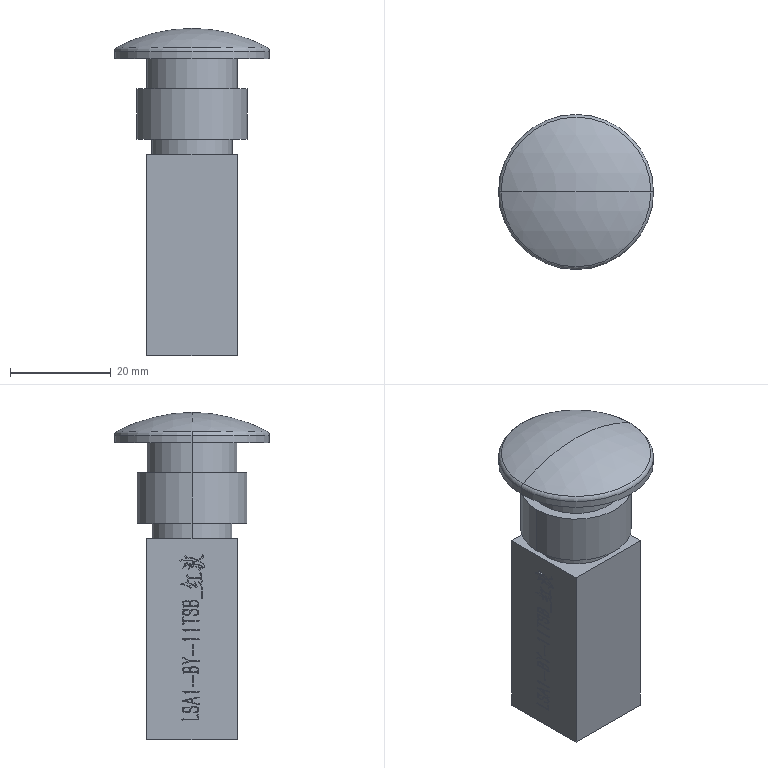Part | STEP file | QA-LSA1-BY-11TSB | 1 solid | 428 faces | box 30.8 x 30.8 x 65 mm | volume 21898 mm3 | plane 279 | spline 137 | cylinder 8 | torus 2 | sphere 2 | commonest cylinder face diameters 16 x2 18 x2 22 x2 30.8 x2